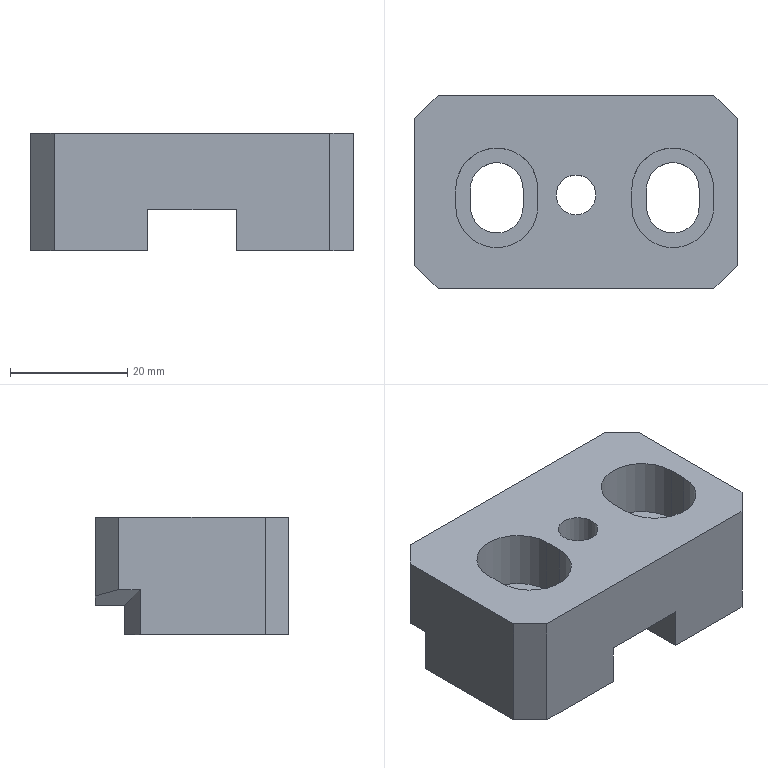Part | NX | features 20 2 | 1 solid | 41 faces | box 55 x 33 x 20 mm | volume 24793 mm3 | plane 32 | cylinder 9 | commonest cylinder face diameters 9 x4 14 x4 6.8 x1
STEP:
#1=CARTESIAN_POINT('',(976.502,-433.5,16.5));
#2=VERTEX_POINT('',#1);
#3=CARTESIAN_POINT('',(962.502,-433.5,16.5));
#4=VERTEX_POINT('',#3);
#5=CARTESIAN_POINT('',(969.502,-433.5,16.5));
#6=DIRECTION('',(0.,0.,1.));
#7=DIRECTION('',(1.,0.,0.));
#8=AXIS2_PLACEMENT_3D('',#5,#6,#7);
#9=CIRCLE('',#8,7.);
#10=EDGE_CURVE('',#2,#4,#9,.T.);
#11=ORIENTED_EDGE('',*,*,#10,.F.);
#12=CARTESIAN_POINT('',(976.502,-436.5,16.5));
#13=VERTEX_POINT('',#12);
#14=CARTESIAN_POINT('',(976.502,-450.5,16.5));
#15=DIRECTION('',(0.,1.,0.));
#16=VECTOR('',#15,1000.);
#17=LINE('',#14,#16);
#18=EDGE_CURVE('',#13,#2,#17,.T.);
#19=ORIENTED_EDGE('',*,*,#18,.F.);
#20=CARTESIAN_POINT('',(962.502,-436.5,16.5));
#21=VERTEX_POINT('',#20);
#22=CARTESIAN_POINT('',(969.502,-436.5,16.5));
#23=DIRECTION('',(0.,0.,1.));
#24=DIRECTION('',(1.,0.,0.));
#25=AXIS2_PLACEMENT_3D('',#22,#23,#24);
#26=CIRCLE('',#25,7.);
#27=EDGE_CURVE('',#21,#13,#26,.T.);
#28=ORIENTED_EDGE('',*,*,#27,.F.);
#29=CARTESIAN_POINT('',(962.502,-450.5,16.5));
#30=DIRECTION('',(0.,-1.,0.));
#31=VECTOR('',#30,1000.);
#32=LINE('',#29,#31);
#33=EDGE_CURVE('',#4,#21,#32,.T.);
#34=ORIENTED_EDGE('',*,*,#33,.F.);
#35=EDGE_LOOP('',(#11,#19,#28,#34));
#36=FACE_BOUND('',#35,.T.);
#37=CARTESIAN_POINT('',(946.502,-436.5,16.5));
#38=VERTEX_POINT('',#37);
#39=CARTESIAN_POINT('',(946.502,-433.5,16.5));
#40=VERTEX_POINT('',#39);
#41=CARTESIAN_POINT('',(946.502,-450.5,16.5));
#42=DIRECTION('',(0.,1.,0.));
#43=VECTOR('',#42,1000.);
#44=LINE('',#41,#43);
#45=EDGE_CURVE('',#38,#40,#44,.T.);
#46=ORIENTED_EDGE('',*,*,#45,.F.);
#47=CARTESIAN_POINT('',(932.502,-436.5,16.5));
#48=VERTEX_POINT('',#47);
#49=CARTESIAN_POINT('',(939.502,-436.5,16.5));
#50=DIRECTION('',(0.,0.,1.));
#51=DIRECTION('',(1.,0.,0.));
#52=AXIS2_PLACEMENT_3D('',#49,#50,#51);
#53=CIRCLE('',#52,7.);
#54=EDGE_CURVE('',#48,#38,#53,.T.);
#55=ORIENTED_EDGE('',*,*,#54,.F.);
#56=CARTESIAN_POINT('',(932.502,-433.5,16.5));
#57=VERTEX_POINT('',#56);
#58=CARTESIAN_POINT('',(932.502,-450.5,16.5));
#59=DIRECTION('',(0.,-1.,0.));
#60=VECTOR('',#59,1000.);
#61=LINE('',#58,#60);
#62=EDGE_CURVE('',#57,#48,#61,.T.);
#63=ORIENTED_EDGE('',*,*,#62,.F.);
#64=CARTESIAN_POINT('',(939.502,-433.5,16.5));
#65=DIRECTION('',(0.,0.,1.));
#66=DIRECTION('',(1.,0.,0.));
#67=AXIS2_PLACEMENT_3D('',#64,#65,#66);
#68=CIRCLE('',#67,7.);
#69=EDGE_CURVE('',#40,#57,#68,.T.);
#70=ORIENTED_EDGE('',*,*,#69,.F.);
#71=EDGE_LOOP('',(#46,#55,#63,#70));
#72=FACE_BOUND('',#71,.T.);
#73=CARTESIAN_POINT('',(976.502,-417.5,16.5));
#74=VERTEX_POINT('',#73);
#75=CARTESIAN_POINT('',(929.502,-417.5,16.5));
#76=VERTEX_POINT('',#75);
#77=CARTESIAN_POINT('',(1043.502,-417.5,16.5));
#78=DIRECTION('',(-1.,0.,0.));
#79=VECTOR('',#78,1000.);
#80=LINE('',#77,#79);
#81=EDGE_CURVE('',#74,#76,#80,.T.);
#82=ORIENTED_EDGE('',*,*,#81,.T.);
#83=CARTESIAN_POINT('',(925.502,-421.5,16.5));
#84=VERTEX_POINT('',#83);
#85=CARTESIAN_POINT('',(925.502,-421.5,16.5));
#86=DIRECTION('',(-0.7071,-0.7071,0.));
#87=VECTOR('',#86,1000.);
#88=LINE('',#85,#87);
#89=EDGE_CURVE('',#76,#84,#88,.T.);
#90=ORIENTED_EDGE('',*,*,#89,.T.);
#91=CARTESIAN_POINT('',(925.502,-446.5,16.5));
#92=VERTEX_POINT('',#91);
#93=CARTESIAN_POINT('',(925.502,-417.5,16.5));
#94=DIRECTION('',(0.,-1.,0.));
#95=VECTOR('',#94,1000.);
#96=LINE('',#93,#95);
#97=EDGE_CURVE('',#84,#92,#96,.T.);
#98=ORIENTED_EDGE('',*,*,#97,.T.);
#99=CARTESIAN_POINT('',(929.502,-450.5,16.5));
#100=VERTEX_POINT('',#99);
#101=CARTESIAN_POINT('',(929.502,-450.5,16.5));
#102=DIRECTION('',(0.7071,-0.7071,0.));
#103=VECTOR('',#102,1000.);
#104=LINE('',#101,#103);
#105=EDGE_CURVE('',#92,#100,#104,.T.);
#106=ORIENTED_EDGE('',*,*,#105,.T.);
#107=CARTESIAN_POINT('',(976.502,-450.5,16.5));
#108=VERTEX_POINT('',#107);
#109=CARTESIAN_POINT('',(963.502,-450.5,16.5));
#110=DIRECTION('',(1.,0.,0.));
#111=VECTOR('',#110,1000.);
#112=LINE('',#109,#111);
#113=EDGE_CURVE('',#100,#108,#112,.T.);
#114=ORIENTED_EDGE('',*,*,#113,.T.);
#115=CARTESIAN_POINT('',(980.502,-446.5,16.5));
#116=VERTEX_POINT('',#115);
#117=CARTESIAN_POINT('',(980.502,-446.5,16.5));
#118=DIRECTION('',(0.7071,0.7071,0.));
#119=VECTOR('',#118,1000.);
#120=LINE('',#117,#119);
#121=EDGE_CURVE('',#108,#116,#120,.T.);
#122=ORIENTED_EDGE('',*,*,#121,.T.);
#123=CARTESIAN_POINT('',(980.502,-421.5,16.5));
#124=VERTEX_POINT('',#123);
#125=CARTESIAN_POINT('',(980.502,-450.5,16.5));
#126=DIRECTION('',(0.,1.,0.));
#127=VECTOR('',#126,1000.);
#128=LINE('',#125,#127);
#129=EDGE_CURVE('',#116,#124,#128,.T.);
#130=ORIENTED_EDGE('',*,*,#129,.T.);
#131=CARTESIAN_POINT('',(976.502,-417.5,16.5));
#132=DIRECTION('',(-0.7071,0.7071,0.));
#133=VECTOR('',#132,1000.);
#134=LINE('',#131,#133);
#135=EDGE_CURVE('',#124,#74,#134,.T.);
#136=ORIENTED_EDGE('',*,*,#135,.T.);
#137=EDGE_LOOP('',(#82,#90,#98,#106,#114,#122,#130,#136));
#138=FACE_BOUND('',#137,.T.);
#139=CARTESIAN_POINT('',(956.402,-434.5,16.5));
#140=VERTEX_POINT('',#139);
#141=CARTESIAN_POINT('',(953.002,-434.5,16.5));
#142=DIRECTION('',(0.,0.,-1.));
#143=DIRECTION('',(1.,0.,0.));
#144=AXIS2_PLACEMENT_3D('',#141,#142,#143);
#145=CIRCLE('',#144,3.4);
#146=EDGE_CURVE('',#140,#140,#145,.T.);
#147=ORIENTED_EDGE('',*,*,#146,.T.);
#148=EDGE_LOOP('',(#147));
#149=FACE_BOUND('',#148,.T.);
#150=CARTESIAN_POINT('',(1043.502,-450.5,16.5));
#151=DIRECTION('',(0.,0.,1.));
#152=DIRECTION('',(-1.,0.,0.));
#153=AXIS2_PLACEMENT_3D('',#150,#151,#152);
#154=PLANE('',#153);
#155=ADVANCED_FACE('',(#36,#72,#138,#149),#154,.T.);
#156=CARTESIAN_POINT('',(965.002,-436.5,6.5));
#157=VERTEX_POINT('',#156);
#158=CARTESIAN_POINT('',(965.002,-433.5,6.5));
#159=VERTEX_POINT('',#158);
#160=CARTESIAN_POINT('',(965.002,-432.5,6.5));
#161=DIRECTION('',(0.,1.,0.));
#162=VECTOR('',#161,1000.);
#163=LINE('',#160,#162);
#164=EDGE_CURVE('',#157,#159,#163,.T.);
#165=ORIENTED_EDGE('',*,*,#164,.T.);
#166=CARTESIAN_POINT('',(974.002,-433.5,6.5));
#167=VERTEX_POINT('',#166);
#168=CARTESIAN_POINT('',(969.502,-433.5,6.5));
#169=DIRECTION('',(0.,0.,-1.));
#170=DIRECTION('',(-1.,0.,0.));
#171=AXIS2_PLACEMENT_3D('',#168,#169,#170);
#172=CIRCLE('',#171,4.5);
#173=EDGE_CURVE('',#159,#167,#172,.T.);
#174=ORIENTED_EDGE('',*,*,#173,.T.);
#175=CARTESIAN_POINT('',(974.002,-436.5,6.5));
#176=VERTEX_POINT('',#175);
#177=CARTESIAN_POINT('',(974.002,-439.5,6.5));
#178=DIRECTION('',(0.,-1.,0.));
#179=VECTOR('',#178,1000.);
#180=LINE('',#177,#179);
#181=EDGE_CURVE('',#167,#176,#180,.T.);
#182=ORIENTED_EDGE('',*,*,#181,.T.);
#183=CARTESIAN_POINT('',(969.502,-436.5,6.5));
#184=DIRECTION('',(0.,0.,-1.));
#185=DIRECTION('',(-1.,0.,0.));
#186=AXIS2_PLACEMENT_3D('',#183,#184,#185);
#187=CIRCLE('',#186,4.5);
#188=EDGE_CURVE('',#176,#157,#187,.T.);
#189=ORIENTED_EDGE('',*,*,#188,.T.);
#190=EDGE_LOOP('',(#165,#174,#182,#189));
#191=FACE_BOUND('',#190,.T.);
#192=CARTESIAN_POINT('',(976.502,-433.5,6.5));
#193=VERTEX_POINT('',#192);
#194=CARTESIAN_POINT('',(962.502,-433.5,6.5));
#195=VERTEX_POINT('',#194);
#196=CARTESIAN_POINT('',(969.502,-433.5,6.5));
#197=DIRECTION('',(0.,0.,1.));
#198=DIRECTION('',(-1.,0.,0.));
#199=AXIS2_PLACEMENT_3D('',#196,#197,#198);
#200=CIRCLE('',#199,7.);
#201=EDGE_CURVE('',#193,#195,#200,.T.);
#202=ORIENTED_EDGE('',*,*,#201,.T.);
#203=CARTESIAN_POINT('',(962.502,-436.5,6.5));
#204=VERTEX_POINT('',#203);
#205=CARTESIAN_POINT('',(962.502,-439.5,6.5));
#206=DIRECTION('',(0.,-1.,0.));
#207=VECTOR('',#206,1000.);
#208=LINE('',#205,#207);
#209=EDGE_CURVE('',#195,#204,#208,.T.);
#210=ORIENTED_EDGE('',*,*,#209,.T.);
#211=CARTESIAN_POINT('',(976.502,-436.5,6.5));
#212=VERTEX_POINT('',#211);
#213=CARTESIAN_POINT('',(969.502,-436.5,6.5));
#214=DIRECTION('',(0.,0.,1.));
#215=DIRECTION('',(-1.,0.,0.));
#216=AXIS2_PLACEMENT_3D('',#213,#214,#215);
#217=CIRCLE('',#216,7.);
#218=EDGE_CURVE('',#204,#212,#217,.T.);
#219=ORIENTED_EDGE('',*,*,#218,.T.);
#220=CARTESIAN_POINT('',(976.502,-432.5,6.5));
#221=DIRECTION('',(0.,1.,0.));
#222=VECTOR('',#221,1000.);
#223=LINE('',#220,#222);
#224=EDGE_CURVE('',#212,#193,#223,.T.);
#225=ORIENTED_EDGE('',*,*,#224,.T.);
#226=EDGE_LOOP('',(#202,#210,#219,#225));
#227=FACE_BOUND('',#226,.T.);
#228=CARTESIAN_POINT('',(969.502,-432.5,6.5));
#229=DIRECTION('',(0.,0.,-1.));
#230=DIRECTION('',(1.,0.,0.));
#231=AXIS2_PLACEMENT_3D('',#228,#229,#230);
#232=PLANE('',#231);
#233=ADVANCED_FACE('',(#191,#227),#232,.F.);
#234=CARTESIAN_POINT('',(970.502,-417.5,1.5));
#235=VERTEX_POINT('',#234);
#236=CARTESIAN_POINT('',(970.502,-422.5,1.5));
#237=VERTEX_POINT('',#236);
#238=CARTESIAN_POINT('',(970.502,-425.18,1.5));
#239=DIRECTION('',(0.,-1.,0.));
#240=VECTOR('',#239,1000.);
#241=LINE('',#238,#240);
#242=EDGE_CURVE('',#235,#237,#241,.T.);
#243=ORIENTED_EDGE('',*,*,#242,.F.);
#244=CARTESIAN_POINT('',(976.502,-417.5,3.108));
#245=VERTEX_POINT('',#244);
#246=CARTESIAN_POINT('',(970.502,-417.5,1.5));
#247=DIRECTION('',(-0.9659,0.,-0.2588));
#248=VECTOR('',#247,1000.);
#249=LINE('',#246,#248);
#250=EDGE_CURVE('',#245,#235,#249,.T.);
#251=ORIENTED_EDGE('',*,*,#250,.F.);
#252=CARTESIAN_POINT('',(980.502,-421.5,4.179));
#253=VERTEX_POINT('',#252);
#254=CARTESIAN_POINT('',(963.451,-404.449,-0.3894));
#255=DIRECTION('',(0.6947,-0.6947,0.1862));
#256=VECTOR('',#255,1000.);
#257=LINE('',#254,#256);
#258=EDGE_CURVE('',#245,#253,#257,.T.);
#259=ORIENTED_EDGE('',*,*,#258,.T.);
#260=CARTESIAN_POINT('',(980.502,-425.18,4.179));
#261=VERTEX_POINT('',#260);
#262=CARTESIAN_POINT('',(980.502,-417.5,4.179));
#263=DIRECTION('',(0.,1.,0.));
#264=VECTOR('',#263,1000.);
#265=LINE('',#262,#264);
#266=EDGE_CURVE('',#261,#253,#265,.T.);
#267=ORIENTED_EDGE('',*,*,#266,.F.);
#268=CARTESIAN_POINT('',(979.875,-425.012,4.011));
#269=DIRECTION('',(0.9351,-0.2506,0.2506));
#270=VECTOR('',#269,1000.);
#271=LINE('',#268,#270);
#272=EDGE_CURVE('',#237,#261,#271,.T.);
#273=ORIENTED_EDGE('',*,*,#272,.F.);
#274=EDGE_LOOP('',(#243,#251,#259,#267,#273));
#275=FACE_BOUND('',#274,.T.);
#276=CARTESIAN_POINT('',(970.502,-396.891,1.5));
#277=DIRECTION('',(0.2588,0.,-0.9659));
#278=DIRECTION('',(0.9659,0.,0.2588));
#279=AXIS2_PLACEMENT_3D('',#276,#277,#278);
#280=PLANE('',#279);
#281=ADVANCED_FACE('',(#275),#280,.T.);
#282=CARTESIAN_POINT('',(944.002,-433.5,6.5));
#283=VERTEX_POINT('',#282);
#284=CARTESIAN_POINT('',(944.002,-436.5,6.5));
#285=VERTEX_POINT('',#284);
#286=CARTESIAN_POINT('',(944.002,-432.5,6.5));
#287=DIRECTION('',(0.,-1.,0.));
#288=VECTOR('',#287,1000.);
#289=LINE('',#286,#288);
#290=EDGE_CURVE('',#283,#285,#289,.T.);
#291=ORIENTED_EDGE('',*,*,#290,.T.);
#292=CARTESIAN_POINT('',(935.002,-436.5,6.5));
#293=VERTEX_POINT('',#292);
#294=CARTESIAN_POINT('',(939.502,-436.5,6.5));
#295=DIRECTION('',(0.,0.,-1.));
#296=DIRECTION('',(-1.,0.,0.));
#297=AXIS2_PLACEMENT_3D('',#294,#295,#296);
#298=CIRCLE('',#297,4.5);
#299=EDGE_CURVE('',#285,#293,#298,.T.);
#300=ORIENTED_EDGE('',*,*,#299,.T.);
#301=CARTESIAN_POINT('',(935.002,-433.5,6.5));
#302=VERTEX_POINT('',#301);
#303=CARTESIAN_POINT('',(935.002,-439.5,6.5));
#304=DIRECTION('',(0.,1.,0.));
#305=VECTOR('',#304,1000.);
#306=LINE('',#303,#305);
#307=EDGE_CURVE('',#293,#302,#306,.T.);
#308=ORIENTED_EDGE('',*,*,#307,.T.);
#309=CARTESIAN_POINT('',(939.502,-433.5,6.5));
#310=DIRECTION('',(0.,0.,-1.));
#311=DIRECTION('',(-1.,0.,0.));
#312=AXIS2_PLACEMENT_3D('',#309,#310,#311);
#313=CIRCLE('',#312,4.5);
#314=EDGE_CURVE('',#302,#283,#313,.T.);
#315=ORIENTED_EDGE('',*,*,#314,.T.);
#316=EDGE_LOOP('',(#291,#300,#308,#315));
#317=FACE_BOUND('',#316,.T.);
#318=CARTESIAN_POINT('',(946.502,-433.5,6.5));
#319=VERTEX_POINT('',#318);
#320=CARTESIAN_POINT('',(932.502,-433.5,6.5));
#321=VERTEX_POINT('',#320);
#322=CARTESIAN_POINT('',(939.502,-433.5,6.5));
#323=DIRECTION('',(0.,0.,1.));
#324=DIRECTION('',(-1.,0.,0.));
#325=AXIS2_PLACEMENT_3D('',#322,#323,#324);
#326=CIRCLE('',#325,7.);
#327=EDGE_CURVE('',#319,#321,#326,.T.);
#328=ORIENTED_EDGE('',*,*,#327,.T.);
#329=CARTESIAN_POINT('',(932.502,-436.5,6.5));
#330=VERTEX_POINT('',#329);
#331=CARTESIAN_POINT('',(932.502,-432.5,6.5));
#332=DIRECTION('',(0.,-1.,0.));
#333=VECTOR('',#332,1000.);
#334=LINE('',#331,#333);
#335=EDGE_CURVE('',#321,#330,#334,.T.);
#336=ORIENTED_EDGE('',*,*,#335,.T.);
#337=CARTESIAN_POINT('',(946.502,-436.5,6.5));
#338=VERTEX_POINT('',#337);
#339=CARTESIAN_POINT('',(939.502,-436.5,6.5));
#340=DIRECTION('',(0.,0.,1.));
#341=DIRECTION('',(-1.,0.,0.));
#342=AXIS2_PLACEMENT_3D('',#339,#340,#341);
#343=CIRCLE('',#342,7.);
#344=EDGE_CURVE('',#330,#338,#343,.T.);
#345=ORIENTED_EDGE('',*,*,#344,.T.);
#346=CARTESIAN_POINT('',(946.502,-439.5,6.5));
#347=DIRECTION('',(0.,1.,0.));
#348=VECTOR('',#347,1000.);
#349=LINE('',#346,#348);
#350=EDGE_CURVE('',#338,#319,#349,.T.);
#351=ORIENTED_EDGE('',*,*,#350,.T.);
#352=EDGE_LOOP('',(#328,#336,#345,#351));
#353=FACE_BOUND('',#352,.T.);
#354=CARTESIAN_POINT('',(939.502,-432.5,6.5));
#355=DIRECTION('',(0.,0.,-1.));
#356=DIRECTION('',(-1.,0.,0.));
#357=AXIS2_PLACEMENT_3D('',#354,#355,#356);
#358=PLANE('',#357);
#359=ADVANCED_FACE('',(#317,#353),#358,.F.);
#360=ORIENTED_EDGE('',*,*,#33,.T.);
#361=CARTESIAN_POINT('',(962.502,-436.5,42.5));
#362=DIRECTION('',(0.,0.,1.));
#363=VECTOR('',#362,1000.);
#364=LINE('',#361,#363);
#365=EDGE_CURVE('',#204,#21,#364,.T.);
#366=ORIENTED_EDGE('',*,*,#365,.F.);
#367=ORIENTED_EDGE('',*,*,#209,.F.);
#368=CARTESIAN_POINT('',(962.502,-433.5,42.5));
#369=DIRECTION('',(0.,0.,1.));
#370=VECTOR('',#369,1000.);
#371=LINE('',#368,#370);
#372=EDGE_CURVE('',#195,#4,#371,.T.);
#373=ORIENTED_EDGE('',*,*,#372,.T.);
#374=EDGE_LOOP('',(#360,#366,#367,#373));
#375=FACE_BOUND('',#374,.T.);
#376=CARTESIAN_POINT('',(962.502,-439.5,42.5));
#377=DIRECTION('',(-1.,0.,0.));
#378=DIRECTION('',(0.,0.,-1.));
#379=AXIS2_PLACEMENT_3D('',#376,#377,#378);
#380=PLANE('',#379);
#381=ADVANCED_FACE('',(#375),#380,.F.);
#382=ORIENTED_EDGE('',*,*,#27,.T.);
#383=CARTESIAN_POINT('',(976.502,-436.5,42.5));
#384=DIRECTION('',(0.,0.,1.));
#385=VECTOR('',#384,1000.);
#386=LINE('',#383,#385);
#387=EDGE_CURVE('',#212,#13,#386,.T.);
#388=ORIENTED_EDGE('',*,*,#387,.F.);
#389=ORIENTED_EDGE('',*,*,#218,.F.);
#390=ORIENTED_EDGE('',*,*,#365,.T.);
#391=EDGE_LOOP('',(#382,#388,#389,#390));
#392=FACE_BOUND('',#391,.T.);
#393=CARTESIAN_POINT('',(969.502,-436.5,42.5));
#394=DIRECTION('',(0.,0.,-1.));
#395=DIRECTION('',(1.,0.,0.));
#396=AXIS2_PLACEMENT_3D('',#393,#394,#395);
#397=CYLINDRICAL_SURFACE('',#396,7.);
#398=ADVANCED_FACE('',(#392),#397,.F.);
#399=ORIENTED_EDGE('',*,*,#18,.T.);
#400=CARTESIAN_POINT('',(976.502,-433.5,42.5));
#401=DIRECTION('',(0.,0.,1.));
#402=VECTOR('',#401,1000.);
#403=LINE('',#400,#402);
#404=EDGE_CURVE('',#193,#2,#403,.T.);
#405=ORIENTED_EDGE('',*,*,#404,.F.);
#406=ORIENTED_EDGE('',*,*,#224,.F.);
#407=ORIENTED_EDGE('',*,*,#387,.T.);
#408=EDGE_LOOP('',(#399,#405,#406,#407));
#409=FACE_BOUND('',#408,.T.);
#410=CARTESIAN_POINT('',(976.502,-432.5,42.5));
#411=DIRECTION('',(1.,0.,0.));
#412=DIRECTION('',(0.,0.,1.));
#413=AXIS2_PLACEMENT_3D('',#410,#411,#412);
#414=PLANE('',#413);
#415=ADVANCED_FACE('',(#409),#414,.F.);
#416=ORIENTED_EDGE('',*,*,#10,.T.);
#417=ORIENTED_EDGE('',*,*,#372,.F.);
#418=ORIENTED_EDGE('',*,*,#201,.F.);
#419=ORIENTED_EDGE('',*,*,#404,.T.);
#420=EDGE_LOOP('',(#416,#417,#418,#419));
#421=FACE_BOUND('',#420,.T.);
#422=CARTESIAN_POINT('',(969.502,-433.5,42.5));
#423=DIRECTION('',(0.,0.,-1.));
#424=DIRECTION('',(1.,0.,0.));
#425=AXIS2_PLACEMENT_3D('',#422,#423,#424);
#426=CYLINDRICAL_SURFACE('',#425,7.);
#427=ADVANCED_FACE('',(#421),#426,.F.);
#428=ORIENTED_EDGE('',*,*,#135,.F.);
#429=CARTESIAN_POINT('',(980.502,-421.5,11.5));
#430=DIRECTION('',(0.,0.,1.));
#431=VECTOR('',#430,1000.);
#432=LINE('',#429,#431);
#433=EDGE_CURVE('',#253,#124,#432,.T.);
#434=ORIENTED_EDGE('',*,*,#433,.F.);
#435=ORIENTED_EDGE('',*,*,#258,.F.);
#436=CARTESIAN_POINT('',(976.502,-417.5,11.5));
#437=DIRECTION('',(0.,0.,-1.));
#438=VECTOR('',#437,1000.);
#439=LINE('',#436,#438);
#440=EDGE_CURVE('',#74,#245,#439,.T.);
#441=ORIENTED_EDGE('',*,*,#440,.F.);
#442=EDGE_LOOP('',(#428,#434,#435,#441));
#443=FACE_BOUND('',#442,.T.);
#444=CARTESIAN_POINT('',(976.502,-417.5,11.5));
#445=DIRECTION('',(-0.7071,-0.7071,0.));
#446=DIRECTION('',(0.,0.,-1.));
#447=AXIS2_PLACEMENT_3D('',#444,#445,#446);
#448=PLANE('',#447);
#449=ADVANCED_FACE('',(#443),#448,.F.);
#450=ORIENTED_EDGE('',*,*,#69,.T.);
#451=CARTESIAN_POINT('',(932.502,-433.5,42.5));
#452=DIRECTION('',(0.,0.,-1.));
#453=VECTOR('',#452,1000.);
#454=LINE('',#451,#453);
#455=EDGE_CURVE('',#57,#321,#454,.T.);
#456=ORIENTED_EDGE('',*,*,#455,.T.);
#457=ORIENTED_EDGE('',*,*,#327,.F.);
#458=CARTESIAN_POINT('',(946.502,-433.5,42.5));
#459=DIRECTION('',(0.,0.,-1.));
#460=VECTOR('',#459,1000.);
#461=LINE('',#458,#460);
#462=EDGE_CURVE('',#40,#319,#461,.T.);
#463=ORIENTED_EDGE('',*,*,#462,.F.);
#464=EDGE_LOOP('',(#450,#456,#457,#463));
#465=FACE_BOUND('',#464,.T.);
#466=CARTESIAN_POINT('',(939.502,-433.5,42.5));
#467=DIRECTION('',(0.,0.,-1.));
#468=DIRECTION('',(-1.,0.,0.));
#469=AXIS2_PLACEMENT_3D('',#466,#467,#468);
#470=CYLINDRICAL_SURFACE('',#469,7.);
#471=ADVANCED_FACE('',(#465),#470,.F.);
#472=ORIENTED_EDGE('',*,*,#62,.T.);
#473=CARTESIAN_POINT('',(932.502,-436.5,42.5));
#474=DIRECTION('',(0.,0.,-1.));
#475=VECTOR('',#474,1000.);
#476=LINE('',#473,#475);
#477=EDGE_CURVE('',#48,#330,#476,.T.);
#478=ORIENTED_EDGE('',*,*,#477,.T.);
#479=ORIENTED_EDGE('',*,*,#335,.F.);
#480=ORIENTED_EDGE('',*,*,#455,.F.);
#481=EDGE_LOOP('',(#472,#478,#479,#480));
#482=FACE_BOUND('',#481,.T.);
#483=CARTESIAN_POINT('',(932.502,-432.5,42.5));
#484=DIRECTION('',(-1.,0.,0.));
#485=DIRECTION('',(0.,0.,1.));
#486=AXIS2_PLACEMENT_3D('',#483,#484,#485);
#487=PLANE('',#486);
#488=ADVANCED_FACE('',(#482),#487,.F.);
#489=ORIENTED_EDGE('',*,*,#54,.T.);
#490=CARTESIAN_POINT('',(946.502,-436.5,42.5));
#491=DIRECTION('',(0.,0.,-1.));
#492=VECTOR('',#491,1000.);
#493=LINE('',#490,#492);
#494=EDGE_CURVE('',#38,#338,#493,.T.);
#495=ORIENTED_EDGE('',*,*,#494,.T.);
#496=ORIENTED_EDGE('',*,*,#344,.F.);
#497=ORIENTED_EDGE('',*,*,#477,.F.);
#498=EDGE_LOOP('',(#489,#495,#496,#497));
#499=FACE_BOUND('',#498,.T.);
#500=CARTESIAN_POINT('',(939.502,-436.5,42.5));
#501=DIRECTION('',(0.,0.,-1.));
#502=DIRECTION('',(-1.,0.,0.));
#503=AXIS2_PLACEMENT_3D('',#500,#501,#502);
#504=CYLINDRICAL_SURFACE('',#503,7.);
#505=ADVANCED_FACE('',(#499),#504,.F.);
#506=ORIENTED_EDGE('',*,*,#45,.T.);
#507=ORIENTED_EDGE('',*,*,#462,.T.);
#508=ORIENTED_EDGE('',*,*,#350,.F.);
#509=ORIENTED_EDGE('',*,*,#494,.F.);
#510=EDGE_LOOP('',(#506,#507,#508,#509));
#511=FACE_BOUND('',#510,.T.);
#512=CARTESIAN_POINT('',(946.502,-439.5,42.5));
#513=DIRECTION('',(1.,0.,0.));
#514=DIRECTION('',(0.,0.,-1.));
#515=AXIS2_PLACEMENT_3D('',#512,#513,#514);
#516=PLANE('',#515);
#517=ADVANCED_FACE('',(#511),#516,.F.);
#518=ORIENTED_EDGE('',*,*,#266,.T.);
#519=ORIENTED_EDGE('',*,*,#433,.T.);
#520=ORIENTED_EDGE('',*,*,#129,.F.);
#521=CARTESIAN_POINT('',(980.502,-446.5,-3.5));
#522=VERTEX_POINT('',#521);
#523=CARTESIAN_POINT('',(980.502,-446.5,11.5));
#524=DIRECTION('',(0.,0.,-1.));
#525=VECTOR('',#524,1000.);
#526=LINE('',#523,#525);
#527=EDGE_CURVE('',#116,#522,#526,.T.);
#528=ORIENTED_EDGE('',*,*,#527,.T.);
#529=CARTESIAN_POINT('',(980.502,-425.18,-3.5));
#530=VERTEX_POINT('',#529);
#531=CARTESIAN_POINT('',(980.502,-450.5,-3.5));
#532=DIRECTION('',(0.,1.,0.));
#533=VECTOR('',#532,1000.);
#534=LINE('',#531,#533);
#535=EDGE_CURVE('',#522,#530,#534,.T.);
#536=ORIENTED_EDGE('',*,*,#535,.T.);
#537=CARTESIAN_POINT('',(980.502,-425.18,3.5));
#538=DIRECTION('',(0.,0.,-1.));
#539=VECTOR('',#538,1000.);
#540=LINE('',#537,#539);
#541=EDGE_CURVE('',#261,#530,#540,.T.);
#542=ORIENTED_EDGE('',*,*,#541,.F.);
#543=EDGE_LOOP('',(#518,#519,#520,#528,#536,#542));
#544=FACE_BOUND('',#543,.T.);
#545=CARTESIAN_POINT('',(980.502,-450.5,11.5));
#546=DIRECTION('',(-1.,0.,0.));
#547=DIRECTION('',(0.,0.,-1.));
#548=AXIS2_PLACEMENT_3D('',#545,#546,#547);
#549=PLANE('',#548);
#550=ADVANCED_FACE('',(#544),#549,.F.);
#551=CARTESIAN_POINT('',(970.501,-422.5,1.5));
#552=VERTEX_POINT('',#551);
#553=CARTESIAN_POINT('',(980.502,-425.18,1.5));
#554=DIRECTION('',(0.9659,-0.2588,0.));
#555=VECTOR('',#554,1000.);
#556=LINE('',#553,#555);
#557=EDGE_CURVE('',#552,#237,#556,.T.);
#558=ORIENTED_EDGE('',*,*,#557,.T.);
#559=ORIENTED_EDGE('',*,*,#272,.T.);
#560=ORIENTED_EDGE('',*,*,#541,.T.);
#561=CARTESIAN_POINT('',(970.501,-422.5,-3.5));
#562=VERTEX_POINT('',#561);
#563=CARTESIAN_POINT('',(980.502,-425.18,-3.5));
#564=DIRECTION('',(-0.9659,0.2588,0.));
#565=VECTOR('',#564,1000.);
#566=LINE('',#563,#565);
#567=EDGE_CURVE('',#530,#562,#566,.T.);
#568=ORIENTED_EDGE('',*,*,#567,.T.);
#569=CARTESIAN_POINT('',(970.501,-422.5,3.5));
#570=DIRECTION('',(0.,0.,1.));
#571=VECTOR('',#570,1000.);
#572=LINE('',#569,#571);
#573=EDGE_CURVE('',#562,#552,#572,.T.);
#574=ORIENTED_EDGE('',*,*,#573,.T.);
#575=EDGE_LOOP('',(#558,#559,#560,#568,#574));
#576=FACE_BOUND('',#575,.T.);
#577=CARTESIAN_POINT('',(980.502,-425.18,3.5));
#578=DIRECTION('',(-0.2588,-0.9659,0.));
#579=DIRECTION('',(0.9659,-0.2588,0.));
#580=AXIS2_PLACEMENT_3D('',#577,#578,#579);
#581=PLANE('',#580);
#582=ADVANCED_FACE('',(#576),#581,.F.);
#583=ORIENTED_EDGE('',*,*,#173,.F.);
#584=CARTESIAN_POINT('',(965.002,-433.5,-3.5));
#585=VERTEX_POINT('',#584);
#586=CARTESIAN_POINT('',(965.002,-433.5,42.5));
#587=DIRECTION('',(0.,0.,1.));
#588=VECTOR('',#587,1000.);
#589=LINE('',#586,#588);
#590=EDGE_CURVE('',#585,#159,#589,.T.);
#591=ORIENTED_EDGE('',*,*,#590,.F.);
#592=CARTESIAN_POINT('',(974.002,-433.5,-3.5));
#593=VERTEX_POINT('',#592);
#594=CARTESIAN_POINT('',(969.502,-433.5,-3.5));
#595=DIRECTION('',(0.,0.,1.));
#596=DIRECTION('',(1.,0.,0.));
#597=AXIS2_PLACEMENT_3D('',#594,#595,#596);
#598=CIRCLE('',#597,4.5);
#599=EDGE_CURVE('',#593,#585,#598,.T.);
#600=ORIENTED_EDGE('',*,*,#599,.F.);
#601=CARTESIAN_POINT('',(974.002,-433.5,42.5));
#602=DIRECTION('',(0.,0.,1.));
#603=VECTOR('',#602,1000.);
#604=LINE('',#601,#603);
#605=EDGE_CURVE('',#593,#167,#604,.T.);
#606=ORIENTED_EDGE('',*,*,#605,.T.);
#607=EDGE_LOOP('',(#583,#591,#600,#606));
#608=FACE_BOUND('',#607,.T.);
#609=CARTESIAN_POINT('',(969.502,-433.5,42.5));
#610=DIRECTION('',(0.,0.,-1.));
#611=DIRECTION('',(1.,0.,0.));
#612=AXIS2_PLACEMENT_3D('',#609,#610,#611);
#613=CYLINDRICAL_SURFACE('',#612,4.5);
#614=ADVANCED_FACE('',(#608),#613,.F.);
#615=ORIENTED_EDGE('',*,*,#181,.F.);
#616=ORIENTED_EDGE('',*,*,#605,.F.);
#617=CARTESIAN_POINT('',(974.002,-436.5,-3.5));
#618=VERTEX_POINT('',#617);
#619=CARTESIAN_POINT('',(974.002,-439.5,-3.5));
#620=DIRECTION('',(0.,1.,0.));
#621=VECTOR('',#620,1000.);
#622=LINE('',#619,#621);
#623=EDGE_CURVE('',#618,#593,#622,.T.);
#624=ORIENTED_EDGE('',*,*,#623,.F.);
#625=CARTESIAN_POINT('',(974.002,-436.5,42.5));
#626=DIRECTION('',(0.,0.,1.));
#627=VECTOR('',#626,1000.);
#628=LINE('',#625,#627);
#629=EDGE_CURVE('',#618,#176,#628,.T.);
#630=ORIENTED_EDGE('',*,*,#629,.T.);
#631=EDGE_LOOP('',(#615,#616,#624,#630));
#632=FACE_BOUND('',#631,.T.);
#633=CARTESIAN_POINT('',(974.002,-439.5,42.5));
#634=DIRECTION('',(-1.,0.,0.));
#635=DIRECTION('',(0.,0.,-1.));
#636=AXIS2_PLACEMENT_3D('',#633,#634,#635);
#637=PLANE('',#636);
#638=ADVANCED_FACE('',(#632),#637,.T.);
#639=ORIENTED_EDGE('',*,*,#188,.F.);
#640=ORIENTED_EDGE('',*,*,#629,.F.);
#641=CARTESIAN_POINT('',(965.002,-436.5,-3.5));
#642=VERTEX_POINT('',#641);
#643=CARTESIAN_POINT('',(969.502,-436.5,-3.5));
#644=DIRECTION('',(0.,0.,1.));
#645=DIRECTION('',(1.,0.,0.));
#646=AXIS2_PLACEMENT_3D('',#643,#644,#645);
#647=CIRCLE('',#646,4.5);
#648=EDGE_CURVE('',#642,#618,#647,.T.);
#649=ORIENTED_EDGE('',*,*,#648,.F.);
#650=CARTESIAN_POINT('',(965.002,-436.5,42.5));
#651=DIRECTION('',(0.,0.,1.));
#652=VECTOR('',#651,1000.);
#653=LINE('',#650,#652);
#654=EDGE_CURVE('',#642,#157,#653,.T.);
#655=ORIENTED_EDGE('',*,*,#654,.T.);
#656=EDGE_LOOP('',(#639,#640,#649,#655));
#657=FACE_BOUND('',#656,.T.);
#658=CARTESIAN_POINT('',(969.502,-436.5,42.5));
#659=DIRECTION('',(0.,0.,-1.));
#660=DIRECTION('',(1.,0.,0.));
#661=AXIS2_PLACEMENT_3D('',#658,#659,#660);
#662=CYLINDRICAL_SURFACE('',#661,4.5);
#663=ADVANCED_FACE('',(#657),#662,.F.);
#664=ORIENTED_EDGE('',*,*,#164,.F.);
#665=ORIENTED_EDGE('',*,*,#654,.F.);
#666=CARTESIAN_POINT('',(965.002,-432.5,-3.5));
#667=DIRECTION('',(0.,-1.,0.));
#668=VECTOR('',#667,1000.);
#669=LINE('',#666,#668);
#670=EDGE_CURVE('',#585,#642,#669,.T.);
#671=ORIENTED_EDGE('',*,*,#670,.F.);
#672=ORIENTED_EDGE('',*,*,#590,.T.);
#673=EDGE_LOOP('',(#664,#665,#671,#672));
#674=FACE_BOUND('',#673,.T.);
#675=CARTESIAN_POINT('',(965.002,-432.5,42.5));
#676=DIRECTION('',(1.,0.,0.));
#677=DIRECTION('',(0.,0.,1.));
#678=AXIS2_PLACEMENT_3D('',#675,#676,#677);
#679=PLANE('',#678);
#680=ADVANCED_FACE('',(#674),#679,.T.);
#681=CARTESIAN_POINT('',(960.502,-422.5,-3.5));
#682=VERTEX_POINT('',#681);
#683=CARTESIAN_POINT('',(960.502,-422.5,1.5));
#684=VERTEX_POINT('',#683);
#685=CARTESIAN_POINT('',(960.502,-422.5,-9.5));
#686=DIRECTION('',(0.,0.,1.));
#687=VECTOR('',#686,1000.);
#688=LINE('',#685,#687);
#689=EDGE_CURVE('',#682,#684,#688,.T.);
#690=ORIENTED_EDGE('',*,*,#689,.T.);
#691=CARTESIAN_POINT('',(895.773,-422.5,1.5));
#692=DIRECTION('',(1.,0.,0.));
#693=VECTOR('',#692,1000.);
#694=LINE('',#691,#693);
#695=EDGE_CURVE('',#684,#552,#694,.T.);
#696=ORIENTED_EDGE('',*,*,#695,.T.);
#697=ORIENTED_EDGE('',*,*,#573,.F.);
#698=CARTESIAN_POINT('',(913.501,-422.5,-3.5));
#699=DIRECTION('',(-1.,0.,0.));
#700=VECTOR('',#699,1000.);
#701=LINE('',#698,#700);
#702=EDGE_CURVE('',#562,#682,#701,.T.);
#703=ORIENTED_EDGE('',*,*,#702,.T.);
#704=EDGE_LOOP('',(#690,#696,#697,#703));
#705=FACE_BOUND('',#704,.T.);
#706=CARTESIAN_POINT('',(913.501,-422.5,3.5));
#707=DIRECTION('',(0.,-1.,0.));
#708=DIRECTION('',(0.,0.,1.));
#709=AXIS2_PLACEMENT_3D('',#706,#707,#708);
#710=PLANE('',#709);
#711=ADVANCED_FACE('',(#705),#710,.F.);
#712=CARTESIAN_POINT('',(960.502,-417.5,1.5));
#713=VERTEX_POINT('',#712);
#714=CARTESIAN_POINT('',(960.502,-436.5,1.5));
#715=DIRECTION('',(0.,1.,0.));
#716=VECTOR('',#715,1000.);
#717=LINE('',#714,#716);
#718=EDGE_CURVE('',#684,#713,#717,.T.);
#719=ORIENTED_EDGE('',*,*,#718,.T.);
#720=CARTESIAN_POINT('',(873.502,-417.5,1.5));
#721=DIRECTION('',(1.,0.,0.));
#722=VECTOR('',#721,1000.);
#723=LINE('',#720,#722);
#724=EDGE_CURVE('',#713,#235,#723,.T.);
#725=ORIENTED_EDGE('',*,*,#724,.T.);
#726=ORIENTED_EDGE('',*,*,#242,.T.);
#727=ORIENTED_EDGE('',*,*,#557,.F.);
#728=ORIENTED_EDGE('',*,*,#695,.F.);
#729=EDGE_LOOP('',(#719,#725,#726,#727,#728));
#730=FACE_BOUND('',#729,.T.);
#731=CARTESIAN_POINT('',(945.773,-396.891,1.5));
#732=DIRECTION('',(0.,0.,-1.));
#733=DIRECTION('',(1.,0.,0.));
#734=AXIS2_PLACEMENT_3D('',#731,#732,#733);
#735=PLANE('',#734);
#736=ADVANCED_FACE('',(#730),#735,.T.);
#737=CARTESIAN_POINT('',(945.502,-417.5,1.5));
#738=VERTEX_POINT('',#737);
#739=CARTESIAN_POINT('',(945.502,-417.5,3.5));
#740=VERTEX_POINT('',#739);
#741=CARTESIAN_POINT('',(945.502,-417.5,11.5));
#742=DIRECTION('',(0.,0.,1.));
#743=VECTOR('',#742,1000.);
#744=LINE('',#741,#743);
#745=EDGE_CURVE('',#738,#740,#744,.T.);
#746=ORIENTED_EDGE('',*,*,#745,.F.);
#747=CARTESIAN_POINT('',(935.502,-417.5,1.5));
#748=VERTEX_POINT('',#747);
#749=CARTESIAN_POINT('',(1021.502,-417.5,1.5));
#750=DIRECTION('',(1.,0.,0.));
#751=VECTOR('',#750,1000.);
#752=LINE('',#749,#751);
#753=EDGE_CURVE('',#748,#738,#752,.T.);
#754=ORIENTED_EDGE('',*,*,#753,.F.);
#755=CARTESIAN_POINT('',(929.502,-417.5,3.108));
#756=VERTEX_POINT('',#755);
#757=CARTESIAN_POINT('',(935.502,-417.5,1.5));
#758=DIRECTION('',(-0.9659,0.,0.2588));
#759=VECTOR('',#758,1000.);
#760=LINE('',#757,#759);
#761=EDGE_CURVE('',#748,#756,#760,.T.);
#762=ORIENTED_EDGE('',*,*,#761,.T.);
#763=CARTESIAN_POINT('',(929.502,-417.5,11.5));
#764=DIRECTION('',(0.,0.,1.));
#765=VECTOR('',#764,1000.);
#766=LINE('',#763,#765);
#767=EDGE_CURVE('',#756,#76,#766,.T.);
#768=ORIENTED_EDGE('',*,*,#767,.T.);
#769=ORIENTED_EDGE('',*,*,#81,.F.);
#770=ORIENTED_EDGE('',*,*,#440,.T.);
#771=ORIENTED_EDGE('',*,*,#250,.T.);
#772=ORIENTED_EDGE('',*,*,#724,.F.);
#773=CARTESIAN_POINT('',(960.502,-417.5,3.5));
#774=VERTEX_POINT('',#773);
#775=CARTESIAN_POINT('',(960.502,-417.5,11.5));
#776=DIRECTION('',(0.,0.,-1.));
#777=VECTOR('',#776,1000.);
#778=LINE('',#775,#777);
#779=EDGE_CURVE('',#774,#713,#778,.T.);
#780=ORIENTED_EDGE('',*,*,#779,.F.);
#781=CARTESIAN_POINT('',(936.002,-417.5,3.5));
#782=DIRECTION('',(1.,0.,0.));
#783=VECTOR('',#782,1000.);
#784=LINE('',#781,#783);
#785=EDGE_CURVE('',#740,#774,#784,.T.);
#786=ORIENTED_EDGE('',*,*,#785,.F.);
#787=EDGE_LOOP('',(#746,#754,#762,#768,#769,#770,#771,#772,#780,#786));
#788=FACE_BOUND('',#787,.T.);
#789=CARTESIAN_POINT('',(1043.502,-417.5,11.5));
#790=DIRECTION('',(0.,-1.,0.));
#791=DIRECTION('',(0.,0.,1.));
#792=AXIS2_PLACEMENT_3D('',#789,#790,#791);
#793=PLANE('',#792);
#794=ADVANCED_FACE('',(#788),#793,.F.);
#795=ORIENTED_EDGE('',*,*,#89,.F.);
#796=ORIENTED_EDGE('',*,*,#767,.F.);
#797=CARTESIAN_POINT('',(925.502,-421.5,4.179));
#798=VERTEX_POINT('',#797);
#799=CARTESIAN_POINT('',(942.554,-404.449,-0.3894));
#800=DIRECTION('',(0.6947,0.6947,-0.1862));
#801=VECTOR('',#800,1000.);
#802=LINE('',#799,#801);
#803=EDGE_CURVE('',#798,#756,#802,.T.);
#804=ORIENTED_EDGE('',*,*,#803,.F.);
#805=CARTESIAN_POINT('',(925.502,-421.5,11.5));
#806=DIRECTION('',(0.,0.,-1.));
#807=VECTOR('',#806,1000.);
#808=LINE('',#805,#807);
#809=EDGE_CURVE('',#84,#798,#808,.T.);
#810=ORIENTED_EDGE('',*,*,#809,.F.);
#811=EDGE_LOOP('',(#795,#796,#804,#810));
#812=FACE_BOUND('',#811,.T.);
#813=CARTESIAN_POINT('',(925.502,-421.5,11.5));
#814=DIRECTION('',(0.7071,-0.7071,0.));
#815=DIRECTION('',(0.,0.,-1.));
#816=AXIS2_PLACEMENT_3D('',#813,#814,#815);
#817=PLANE('',#816);
#818=ADVANCED_FACE('',(#812),#817,.F.);
#819=ORIENTED_EDGE('',*,*,#299,.F.);
#820=CARTESIAN_POINT('',(944.002,-436.5,-3.5));
#821=VERTEX_POINT('',#820);
#822=CARTESIAN_POINT('',(944.002,-436.5,42.5));
#823=DIRECTION('',(0.,0.,-1.));
#824=VECTOR('',#823,1000.);
#825=LINE('',#822,#824);
#826=EDGE_CURVE('',#285,#821,#825,.T.);
#827=ORIENTED_EDGE('',*,*,#826,.T.);
#828=CARTESIAN_POINT('',(935.002,-436.5,-3.5));
#829=VERTEX_POINT('',#828);
#830=CARTESIAN_POINT('',(939.502,-436.5,-3.5));
#831=DIRECTION('',(0.,0.,-1.));
#832=DIRECTION('',(1.,0.,0.));
#833=AXIS2_PLACEMENT_3D('',#830,#831,#832);
#834=CIRCLE('',#833,4.5);
#835=EDGE_CURVE('',#821,#829,#834,.T.);
#836=ORIENTED_EDGE('',*,*,#835,.T.);
#837=CARTESIAN_POINT('',(935.002,-436.5,42.5));
#838=DIRECTION('',(0.,0.,-1.));
#839=VECTOR('',#838,1000.);
#840=LINE('',#837,#839);
#841=EDGE_CURVE('',#293,#829,#840,.T.);
#842=ORIENTED_EDGE('',*,*,#841,.F.);
#843=EDGE_LOOP('',(#819,#827,#836,#842));
#844=FACE_BOUND('',#843,.T.);
#845=CARTESIAN_POINT('',(939.502,-436.5,42.5));
#846=DIRECTION('',(0.,0.,-1.));
#847=DIRECTION('',(-1.,0.,0.));
#848=AXIS2_PLACEMENT_3D('',#845,#846,#847);
#849=CYLINDRICAL_SURFACE('',#848,4.5);
#850=ADVANCED_FACE('',(#844),#849,.F.);
#851=ORIENTED_EDGE('',*,*,#307,.F.);
#852=ORIENTED_EDGE('',*,*,#841,.T.);
#853=CARTESIAN_POINT('',(935.002,-433.5,-3.5));
#854=VERTEX_POINT('',#853);
#855=CARTESIAN_POINT('',(935.002,-450.5,-3.5));
#856=DIRECTION('',(0.,1.,0.));
#857=VECTOR('',#856,1000.);
#858=LINE('',#855,#857);
#859=EDGE_CURVE('',#829,#854,#858,.T.);
#860=ORIENTED_EDGE('',*,*,#859,.T.);
#861=CARTESIAN_POINT('',(935.002,-433.5,42.5));
#862=DIRECTION('',(0.,0.,-1.));
#863=VECTOR('',#862,1000.);
#864=LINE('',#861,#863);
#865=EDGE_CURVE('',#302,#854,#864,.T.);
#866=ORIENTED_EDGE('',*,*,#865,.F.);
#867=EDGE_LOOP('',(#851,#852,#860,#866));
#868=FACE_BOUND('',#867,.T.);
#869=CARTESIAN_POINT('',(935.002,-439.5,42.5));
#870=DIRECTION('',(1.,0.,0.));
#871=DIRECTION('',(0.,0.,-1.));
#872=AXIS2_PLACEMENT_3D('',#869,#870,#871);
#873=PLANE('',#872);
#874=ADVANCED_FACE('',(#868),#873,.T.);
#875=ORIENTED_EDGE('',*,*,#314,.F.);
#876=ORIENTED_EDGE('',*,*,#865,.T.);
#877=CARTESIAN_POINT('',(944.002,-433.5,-3.5));
#878=VERTEX_POINT('',#877);
#879=CARTESIAN_POINT('',(939.502,-433.5,-3.5));
#880=DIRECTION('',(0.,0.,-1.));
#881=DIRECTION('',(1.,0.,0.));
#882=AXIS2_PLACEMENT_3D('',#879,#880,#881);
#883=CIRCLE('',#882,4.5);
#884=EDGE_CURVE('',#854,#878,#883,.T.);
#885=ORIENTED_EDGE('',*,*,#884,.T.);
#886=CARTESIAN_POINT('',(944.002,-433.5,42.5));
#887=DIRECTION('',(0.,0.,-1.));
#888=VECTOR('',#887,1000.);
#889=LINE('',#886,#888);
#890=EDGE_CURVE('',#283,#878,#889,.T.);
#891=ORIENTED_EDGE('',*,*,#890,.F.);
#892=EDGE_LOOP('',(#875,#876,#885,#891));
#893=FACE_BOUND('',#892,.T.);
#894=CARTESIAN_POINT('',(939.502,-433.5,42.5));
#895=DIRECTION('',(0.,0.,-1.));
#896=DIRECTION('',(-1.,0.,0.));
#897=AXIS2_PLACEMENT_3D('',#894,#895,#896);
#898=CYLINDRICAL_SURFACE('',#897,4.5);
#899=ADVANCED_FACE('',(#893),#898,.F.);
#900=ORIENTED_EDGE('',*,*,#290,.F.);
#901=ORIENTED_EDGE('',*,*,#890,.T.);
#902=CARTESIAN_POINT('',(944.002,-450.5,-3.5));
#903=DIRECTION('',(0.,-1.,0.));
#904=VECTOR('',#903,1000.);
#905=LINE('',#902,#904);
#906=EDGE_CURVE('',#878,#821,#905,.T.);
#907=ORIENTED_EDGE('',*,*,#906,.T.);
#908=ORIENTED_EDGE('',*,*,#826,.F.);
#909=EDGE_LOOP('',(#900,#901,#907,#908));
#910=FACE_BOUND('',#909,.T.);
#911=CARTESIAN_POINT('',(944.002,-432.5,42.5));
#912=DIRECTION('',(-1.,0.,0.));
#913=DIRECTION('',(0.,0.,1.));
#914=AXIS2_PLACEMENT_3D('',#911,#912,#913);
#915=PLANE('',#914);
#916=ADVANCED_FACE('',(#910),#915,.T.);
#917=ORIENTED_EDGE('',*,*,#97,.F.);
#918=ORIENTED_EDGE('',*,*,#809,.T.);
#919=CARTESIAN_POINT('',(925.502,-425.179,4.179));
#920=VERTEX_POINT('',#919);
#921=CARTESIAN_POINT('',(925.502,-425.179,4.179));
#922=DIRECTION('',(0.,-1.,0.));
#923=VECTOR('',#922,1000.);
#924=LINE('',#921,#923);
#925=EDGE_CURVE('',#798,#920,#924,.T.);
#926=ORIENTED_EDGE('',*,*,#925,.T.);
#927=CARTESIAN_POINT('',(925.502,-425.179,-3.5));
#928=VERTEX_POINT('',#927);
#929=CARTESIAN_POINT('',(925.502,-425.179,3.5));
#930=DIRECTION('',(0.,0.,-1.));
#931=VECTOR('',#930,1000.);
#932=LINE('',#929,#931);
#933=EDGE_CURVE('',#920,#928,#932,.T.);
#934=ORIENTED_EDGE('',*,*,#933,.T.);
#935=CARTESIAN_POINT('',(925.502,-446.5,-3.5));
#936=VERTEX_POINT('',#935);
#937=CARTESIAN_POINT('',(925.502,-417.5,-3.5));
#938=DIRECTION('',(0.,-1.,0.));
#939=VECTOR('',#938,1000.);
#940=LINE('',#937,#939);
#941=EDGE_CURVE('',#928,#936,#940,.T.);
#942=ORIENTED_EDGE('',*,*,#941,.T.);
#943=CARTESIAN_POINT('',(925.502,-446.5,11.5));
#944=DIRECTION('',(0.,0.,1.));
#945=VECTOR('',#944,1000.);
#946=LINE('',#943,#945);
#947=EDGE_CURVE('',#936,#92,#946,.T.);
#948=ORIENTED_EDGE('',*,*,#947,.T.);
#949=EDGE_LOOP('',(#917,#918,#926,#934,#942,#948));
#950=FACE_BOUND('',#949,.T.);
#951=CARTESIAN_POINT('',(925.502,-417.5,11.5));
#952=DIRECTION('',(1.,0.,0.));
#953=DIRECTION('',(0.,0.,1.));
#954=AXIS2_PLACEMENT_3D('',#951,#952,#953);
#955=PLANE('',#954);
#956=ADVANCED_FACE('',(#950),#955,.F.);
#957=ORIENTED_EDGE('',*,*,#925,.F.);
#958=ORIENTED_EDGE('',*,*,#803,.T.);
#959=ORIENTED_EDGE('',*,*,#761,.F.);
#960=CARTESIAN_POINT('',(935.502,-422.5,1.5));
#961=VERTEX_POINT('',#960);
#962=CARTESIAN_POINT('',(935.502,-417.5,1.5));
#963=DIRECTION('',(0.,1.,0.));
#964=VECTOR('',#963,1000.);
#965=LINE('',#962,#964);
#966=EDGE_CURVE('',#961,#748,#965,.T.);
#967=ORIENTED_EDGE('',*,*,#966,.F.);
#968=CARTESIAN_POINT('',(935.501,-422.5,1.5));
#969=VERTEX_POINT('',#968);
#970=CARTESIAN_POINT('',(935.502,-422.5,1.5));
#971=DIRECTION('',(0.9659,0.,-0.2588));
#972=VECTOR('',#971,1000.);
#973=LINE('',#970,#972);
#974=EDGE_CURVE('',#969,#961,#973,.T.);
#975=ORIENTED_EDGE('',*,*,#974,.F.);
#976=CARTESIAN_POINT('',(935.501,-422.5,1.5));
#977=DIRECTION('',(0.9351,0.2506,-0.2506));
#978=VECTOR('',#977,1000.);
#979=LINE('',#976,#978);
#980=EDGE_CURVE('',#920,#969,#979,.T.);
#981=ORIENTED_EDGE('',*,*,#980,.F.);
#982=EDGE_LOOP('',(#957,#958,#959,#967,#975,#981));
#983=FACE_BOUND('',#982,.T.);
#984=CARTESIAN_POINT('',(935.502,-396.891,1.5));
#985=DIRECTION('',(-0.2588,0.,-0.9659));
#986=DIRECTION('',(0.9659,0.,-0.2588));
#987=AXIS2_PLACEMENT_3D('',#984,#985,#986);
#988=PLANE('',#987);
#989=ADVANCED_FACE('',(#983),#988,.T.);
#990=CARTESIAN_POINT('',(935.501,-422.5,-3.5));
#991=VERTEX_POINT('',#990);
#992=CARTESIAN_POINT('',(935.501,-422.5,-3.5));
#993=DIRECTION('',(-0.9659,-0.2588,0.));
#994=VECTOR('',#993,1000.);
#995=LINE('',#992,#994);
#996=EDGE_CURVE('',#991,#928,#995,.T.);
#997=ORIENTED_EDGE('',*,*,#996,.T.);
#998=ORIENTED_EDGE('',*,*,#933,.F.);
#999=ORIENTED_EDGE('',*,*,#980,.T.);
#1000=CARTESIAN_POINT('',(935.501,-422.5,3.5));
#1001=DIRECTION('',(0.,0.,1.));
#1002=VECTOR('',#1001,1000.);
#1003=LINE('',#1000,#1002);
#1004=EDGE_CURVE('',#991,#969,#1003,.T.);
#1005=ORIENTED_EDGE('',*,*,#1004,.F.);
#1006=EDGE_LOOP('',(#997,#998,#999,#1005));
#1007=FACE_BOUND('',#1006,.T.);
#1008=CARTESIAN_POINT('',(935.501,-422.5,3.5));
#1009=DIRECTION('',(0.2588,-0.9659,0.));
#1010=DIRECTION('',(0.9659,0.2588,0.));
#1011=AXIS2_PLACEMENT_3D('',#1008,#1009,#1010);
#1012=PLANE('',#1011);
#1013=ADVANCED_FACE('',(#1007),#1012,.F.);
#1014=ORIENTED_EDGE('',*,*,#996,.F.);
#1015=CARTESIAN_POINT('',(945.502,-422.5,-3.5));
#1016=VERTEX_POINT('',#1015);
#1017=CARTESIAN_POINT('',(981.501,-422.5,-3.5));
#1018=DIRECTION('',(-1.,0.,0.));
#1019=VECTOR('',#1018,1000.);
#1020=LINE('',#1017,#1019);
#1021=EDGE_CURVE('',#1016,#991,#1020,.T.);
#1022=ORIENTED_EDGE('',*,*,#1021,.F.);
#1023=CARTESIAN_POINT('',(945.502,-450.5,-3.5));
#1024=VERTEX_POINT('',#1023);
#1025=CARTESIAN_POINT('',(945.502,-450.5,-3.5));
#1026=DIRECTION('',(0.,-1.,0.));
#1027=VECTOR('',#1026,1000.);
#1028=LINE('',#1025,#1027);
#1029=EDGE_CURVE('',#1016,#1024,#1028,.T.);
#1030=ORIENTED_EDGE('',*,*,#1029,.T.);
#1031=CARTESIAN_POINT('',(929.502,-450.5,-3.5));
#1032=VERTEX_POINT('',#1031);
#1033=CARTESIAN_POINT('',(1003.502,-450.5,-3.5));
#1034=DIRECTION('',(1.,0.,0.));
#1035=VECTOR('',#1034,1000.);
#1036=LINE('',#1033,#1035);
#1037=EDGE_CURVE('',#1032,#1024,#1036,.T.);
#1038=ORIENTED_EDGE('',*,*,#1037,.F.);
#1039=CARTESIAN_POINT('',(929.502,-450.5,-3.5));
#1040=DIRECTION('',(-0.7071,0.7071,0.));
#1041=VECTOR('',#1040,1000.);
#1042=LINE('',#1039,#1041);
#1043=EDGE_CURVE('',#1032,#936,#1042,.T.);
#1044=ORIENTED_EDGE('',*,*,#1043,.T.);
#1045=ORIENTED_EDGE('',*,*,#941,.F.);
#1046=EDGE_LOOP('',(#1014,#1022,#1030,#1038,#1044,#1045));
#1047=FACE_BOUND('',#1046,.T.);
#1048=ORIENTED_EDGE('',*,*,#906,.F.);
#1049=ORIENTED_EDGE('',*,*,#884,.F.);
#1050=ORIENTED_EDGE('',*,*,#859,.F.);
#1051=ORIENTED_EDGE('',*,*,#835,.F.);
#1052=EDGE_LOOP('',(#1048,#1049,#1050,#1051));
#1053=FACE_BOUND('',#1052,.T.);
#1054=CARTESIAN_POINT('',(1073.502,-450.5,-3.5));
#1055=DIRECTION('',(0.,0.,1.));
#1056=DIRECTION('',(-1.,0.,0.));
#1057=AXIS2_PLACEMENT_3D('',#1054,#1055,#1056);
#1058=PLANE('',#1057);
#1059=ADVANCED_FACE('',(#1047,#1053),#1058,.F.);
#1060=ORIENTED_EDGE('',*,*,#1043,.F.);
#1061=CARTESIAN_POINT('',(929.502,-450.5,11.5));
#1062=DIRECTION('',(0.,0.,-1.));
#1063=VECTOR('',#1062,1000.);
#1064=LINE('',#1061,#1063);
#1065=EDGE_CURVE('',#100,#1032,#1064,.T.);
#1066=ORIENTED_EDGE('',*,*,#1065,.F.);
#1067=ORIENTED_EDGE('',*,*,#105,.F.);
#1068=ORIENTED_EDGE('',*,*,#947,.F.);
#1069=EDGE_LOOP('',(#1060,#1066,#1067,#1068));
#1070=FACE_BOUND('',#1069,.T.);
#1071=CARTESIAN_POINT('',(929.502,-450.5,11.5));
#1072=DIRECTION('',(0.7071,0.7071,0.));
#1073=DIRECTION('',(0.,0.,-1.));
#1074=AXIS2_PLACEMENT_3D('',#1071,#1072,#1073);
#1075=PLANE('',#1074);
#1076=ADVANCED_FACE('',(#1070),#1075,.F.);
#1077=CARTESIAN_POINT('',(976.502,-450.5,-3.5));
#1078=VERTEX_POINT('',#1077);
#1079=CARTESIAN_POINT('',(980.502,-446.5,-3.5));
#1080=DIRECTION('',(-0.7071,-0.7071,0.));
#1081=VECTOR('',#1080,1000.);
#1082=LINE('',#1079,#1081);
#1083=EDGE_CURVE('',#522,#1078,#1082,.T.);
#1084=ORIENTED_EDGE('',*,*,#1083,.F.);
#1085=ORIENTED_EDGE('',*,*,#527,.F.);
#1086=ORIENTED_EDGE('',*,*,#121,.F.);
#1087=CARTESIAN_POINT('',(976.502,-450.5,11.5));
#1088=DIRECTION('',(0.,0.,1.));
#1089=VECTOR('',#1088,1000.);
#1090=LINE('',#1087,#1089);
#1091=EDGE_CURVE('',#1078,#108,#1090,.T.);
#1092=ORIENTED_EDGE('',*,*,#1091,.F.);
#1093=EDGE_LOOP('',(#1084,#1085,#1086,#1092));
#1094=FACE_BOUND('',#1093,.T.);
#1095=CARTESIAN_POINT('',(980.502,-446.5,11.5));
#1096=DIRECTION('',(-0.7071,0.7071,0.));
#1097=DIRECTION('',(0.,0.,-1.));
#1098=AXIS2_PLACEMENT_3D('',#1095,#1096,#1097);
#1099=PLANE('',#1098);
#1100=ADVANCED_FACE('',(#1094),#1099,.F.);
#1101=ORIENTED_EDGE('',*,*,#670,.T.);
#1102=ORIENTED_EDGE('',*,*,#648,.T.);
#1103=ORIENTED_EDGE('',*,*,#623,.T.);
#1104=ORIENTED_EDGE('',*,*,#599,.T.);
#1105=EDGE_LOOP('',(#1101,#1102,#1103,#1104));
#1106=FACE_BOUND('',#1105,.T.);
#1107=ORIENTED_EDGE('',*,*,#702,.F.);
#1108=ORIENTED_EDGE('',*,*,#567,.F.);
#1109=ORIENTED_EDGE('',*,*,#535,.F.);
#1110=ORIENTED_EDGE('',*,*,#1083,.T.);
#1111=CARTESIAN_POINT('',(960.502,-450.5,-3.5));
#1112=VERTEX_POINT('',#1111);
#1113=CARTESIAN_POINT('',(843.502,-450.5,-3.5));
#1114=DIRECTION('',(1.,0.,0.));
#1115=VECTOR('',#1114,1000.);
#1116=LINE('',#1113,#1115);
#1117=EDGE_CURVE('',#1112,#1078,#1116,.T.);
#1118=ORIENTED_EDGE('',*,*,#1117,.F.);
#1119=CARTESIAN_POINT('',(960.502,-450.5,-3.5));
#1120=DIRECTION('',(0.,1.,0.));
#1121=VECTOR('',#1120,1000.);
#1122=LINE('',#1119,#1121);
#1123=EDGE_CURVE('',#1112,#682,#1122,.T.);
#1124=ORIENTED_EDGE('',*,*,#1123,.T.);
#1125=EDGE_LOOP('',(#1107,#1108,#1109,#1110,#1118,#1124));
#1126=FACE_BOUND('',#1125,.T.);
#1127=CARTESIAN_POINT('',(863.502,-450.5,-3.5));
#1128=DIRECTION('',(0.,0.,1.));
#1129=DIRECTION('',(-1.,0.,0.));
#1130=AXIS2_PLACEMENT_3D('',#1127,#1128,#1129);
#1131=PLANE('',#1130);
#1132=ADVANCED_FACE('',(#1106,#1126),#1131,.F.);
#1133=ORIENTED_EDGE('',*,*,#1123,.F.);
#1134=CARTESIAN_POINT('',(960.502,-450.5,3.5));
#1135=VERTEX_POINT('',#1134);
#1136=CARTESIAN_POINT('',(960.502,-450.5,-9.5));
#1137=DIRECTION('',(0.,0.,1.));
#1138=VECTOR('',#1137,1000.);
#1139=LINE('',#1136,#1138);
#1140=EDGE_CURVE('',#1112,#1135,#1139,.T.);
#1141=ORIENTED_EDGE('',*,*,#1140,.T.);
#1142=CARTESIAN_POINT('',(960.502,-436.5,3.5));
#1143=DIRECTION('',(0.,-1.,0.));
#1144=VECTOR('',#1143,1000.);
#1145=LINE('',#1142,#1144);
#1146=EDGE_CURVE('',#774,#1135,#1145,.T.);
#1147=ORIENTED_EDGE('',*,*,#1146,.F.);
#1148=ORIENTED_EDGE('',*,*,#779,.T.);
#1149=ORIENTED_EDGE('',*,*,#718,.F.);
#1150=ORIENTED_EDGE('',*,*,#689,.F.);
#1151=EDGE_LOOP('',(#1133,#1141,#1147,#1148,#1149,#1150));
#1152=FACE_BOUND('',#1151,.T.);
#1153=CARTESIAN_POINT('',(960.502,-436.5,-9.5));
#1154=DIRECTION('',(1.,0.,0.));
#1155=DIRECTION('',(0.,0.,-1.));
#1156=AXIS2_PLACEMENT_3D('',#1153,#1154,#1155);
#1157=PLANE('',#1156);
#1158=ADVANCED_FACE('',(#1152),#1157,.F.);
#1159=CARTESIAN_POINT('',(956.402,-434.5,3.5));
#1160=VERTEX_POINT('',#1159);
#1161=CARTESIAN_POINT('',(953.002,-434.5,3.5));
#1162=DIRECTION('',(0.,0.,1.));
#1163=DIRECTION('',(1.,0.,0.));
#1164=AXIS2_PLACEMENT_3D('',#1161,#1162,#1163);
#1165=CIRCLE('',#1164,3.4);
#1166=EDGE_CURVE('',#1160,#1160,#1165,.T.);
#1167=ORIENTED_EDGE('',*,*,#1166,.T.);
#1168=EDGE_LOOP('',(#1167));
#1169=FACE_BOUND('',#1168,.T.);
#1170=CARTESIAN_POINT('',(945.502,-450.5,3.5));
#1171=VERTEX_POINT('',#1170);
#1172=CARTESIAN_POINT('',(856.002,-450.5,3.5));
#1173=DIRECTION('',(1.,0.,0.));
#1174=VECTOR('',#1173,1000.);
#1175=LINE('',#1172,#1174);
#1176=EDGE_CURVE('',#1171,#1135,#1175,.T.);
#1177=ORIENTED_EDGE('',*,*,#1176,.F.);
#1178=CARTESIAN_POINT('',(945.502,-436.5,3.5));
#1179=DIRECTION('',(0.,1.,0.));
#1180=VECTOR('',#1179,1000.);
#1181=LINE('',#1178,#1180);
#1182=EDGE_CURVE('',#1171,#740,#1181,.T.);
#1183=ORIENTED_EDGE('',*,*,#1182,.T.);
#1184=ORIENTED_EDGE('',*,*,#785,.T.);
#1185=ORIENTED_EDGE('',*,*,#1146,.T.);
#1186=EDGE_LOOP('',(#1177,#1183,#1184,#1185));
#1187=FACE_BOUND('',#1186,.T.);
#1188=CARTESIAN_POINT('',(953.002,-436.5,3.5));
#1189=DIRECTION('',(0.,0.,1.));
#1190=DIRECTION('',(0.,-1.,0.));
#1191=AXIS2_PLACEMENT_3D('',#1188,#1189,#1190);
#1192=PLANE('',#1191);
#1193=ADVANCED_FACE('',(#1169,#1187),#1192,.F.);
#1194=ORIENTED_EDGE('',*,*,#1182,.F.);
#1195=CARTESIAN_POINT('',(945.502,-450.5,11.5));
#1196=DIRECTION('',(0.,0.,1.));
#1197=VECTOR('',#1196,1000.);
#1198=LINE('',#1195,#1197);
#1199=EDGE_CURVE('',#1024,#1171,#1198,.T.);
#1200=ORIENTED_EDGE('',*,*,#1199,.F.);
#1201=ORIENTED_EDGE('',*,*,#1029,.F.);
#1202=CARTESIAN_POINT('',(945.502,-422.5,1.5));
#1203=VERTEX_POINT('',#1202);
#1204=CARTESIAN_POINT('',(945.502,-422.5,3.5));
#1205=DIRECTION('',(0.,0.,-1.));
#1206=VECTOR('',#1205,1000.);
#1207=LINE('',#1204,#1206);
#1208=EDGE_CURVE('',#1203,#1016,#1207,.T.);
#1209=ORIENTED_EDGE('',*,*,#1208,.F.);
#1210=CARTESIAN_POINT('',(945.502,-396.891,1.5));
#1211=DIRECTION('',(0.,1.,0.));
#1212=VECTOR('',#1211,1000.);
#1213=LINE('',#1210,#1212);
#1214=EDGE_CURVE('',#1203,#738,#1213,.T.);
#1215=ORIENTED_EDGE('',*,*,#1214,.T.);
#1216=ORIENTED_EDGE('',*,*,#745,.T.);
#1217=EDGE_LOOP('',(#1194,#1200,#1201,#1209,#1215,#1216));
#1218=FACE_BOUND('',#1217,.T.);
#1219=CARTESIAN_POINT('',(945.502,-436.5,0.));
#1220=DIRECTION('',(1.,0.,0.));
#1221=DIRECTION('',(0.,0.,1.));
#1222=AXIS2_PLACEMENT_3D('',#1219,#1220,#1221);
#1223=PLANE('',#1222);
#1224=ADVANCED_FACE('',(#1218),#1223,.T.);
#1225=ORIENTED_EDGE('',*,*,#1037,.T.);
#1226=ORIENTED_EDGE('',*,*,#1199,.T.);
#1227=ORIENTED_EDGE('',*,*,#1176,.T.);
#1228=ORIENTED_EDGE('',*,*,#1140,.F.);
#1229=ORIENTED_EDGE('',*,*,#1117,.T.);
#1230=ORIENTED_EDGE('',*,*,#1091,.T.);
#1231=ORIENTED_EDGE('',*,*,#113,.F.);
#1232=ORIENTED_EDGE('',*,*,#1065,.T.);
#1233=EDGE_LOOP('',(#1225,#1226,#1227,#1228,#1229,#1230,#1231,#1232));
#1234=FACE_BOUND('',#1233,.T.);
#1235=CARTESIAN_POINT('',(963.502,-450.5,11.5));
#1236=DIRECTION('',(0.,1.,0.));
#1237=DIRECTION('',(0.,0.,-1.));
#1238=AXIS2_PLACEMENT_3D('',#1235,#1236,#1237);
#1239=PLANE('',#1238);
#1240=ADVANCED_FACE('',(#1234),#1239,.F.);
#1241=ORIENTED_EDGE('',*,*,#753,.T.);
#1242=ORIENTED_EDGE('',*,*,#1214,.F.);
#1243=CARTESIAN_POINT('',(1011.501,-422.5,1.5));
#1244=DIRECTION('',(1.,0.,0.));
#1245=VECTOR('',#1244,1000.);
#1246=LINE('',#1243,#1245);
#1247=EDGE_CURVE('',#961,#1203,#1246,.T.);
#1248=ORIENTED_EDGE('',*,*,#1247,.F.);
#1249=ORIENTED_EDGE('',*,*,#966,.T.);
#1250=EDGE_LOOP('',(#1241,#1242,#1248,#1249));
#1251=FACE_BOUND('',#1250,.T.);
#1252=CARTESIAN_POINT('',(1043.773,-396.891,1.5));
#1253=DIRECTION('',(0.,0.,-1.));
#1254=DIRECTION('',(1.,0.,0.));
#1255=AXIS2_PLACEMENT_3D('',#1252,#1253,#1254);
#1256=PLANE('',#1255);
#1257=ADVANCED_FACE('',(#1251),#1256,.T.);
#1258=ORIENTED_EDGE('',*,*,#1247,.T.);
#1259=ORIENTED_EDGE('',*,*,#1208,.T.);
#1260=ORIENTED_EDGE('',*,*,#1021,.T.);
#1261=ORIENTED_EDGE('',*,*,#1004,.T.);
#1262=ORIENTED_EDGE('',*,*,#974,.T.);
#1263=EDGE_LOOP('',(#1258,#1259,#1260,#1261,#1262));
#1264=FACE_BOUND('',#1263,.T.);
#1265=CARTESIAN_POINT('',(1011.501,-422.5,3.5));
#1266=DIRECTION('',(0.,-1.,0.));
#1267=DIRECTION('',(0.,0.,1.));
#1268=AXIS2_PLACEMENT_3D('',#1265,#1266,#1267);
#1269=PLANE('',#1268);
#1270=ADVANCED_FACE('',(#1264),#1269,.F.);
#1271=ORIENTED_EDGE('',*,*,#146,.F.);
#1272=EDGE_LOOP('',(#1271));
#1273=FACE_BOUND('',#1272,.T.);
#1274=ORIENTED_EDGE('',*,*,#1166,.F.);
#1275=EDGE_LOOP('',(#1274));
#1276=FACE_BOUND('',#1275,.T.);
#1277=CARTESIAN_POINT('',(953.002,-434.5,16.5));
#1278=DIRECTION('',(0.,0.,-1.));
#1279=DIRECTION('',(-1.,0.,0.));
#1280=AXIS2_PLACEMENT_3D('',#1277,#1278,#1279);
#1281=CYLINDRICAL_SURFACE('',#1280,3.4);
#1282=ADVANCED_FACE('',(#1273,#1276),#1281,.F.);
#1283=CLOSED_SHELL('',(#155,#233,#281,#359,#381,#398,#415,#427,#449,#471,#488,#505,#517,#550,#582,#614,#638,#663,#680,#711,#736,#794,#818,#850,#874,#899,#916,#956,#989,#1013,#1059,#1076,#1100,#1132,#1158,#1193,#1224,#1240,#1257,#1270,#1282));
#1284=MANIFOLD_SOLID_BREP('',#1283);
#1285=(LENGTH_UNIT()NAMED_UNIT(*)SI_UNIT(.MILLI.,.METRE.));
#1286=UNCERTAINTY_MEASURE_WITH_UNIT(LENGTH_MEASURE(0.00001),#1285,'','');
#1287=(NAMED_UNIT(*)PLANE_ANGLE_UNIT()SI_UNIT($,.RADIAN.));
#1288=(NAMED_UNIT(*)SI_UNIT($,.STERADIAN.)SOLID_ANGLE_UNIT());
#1289=(GEOMETRIC_REPRESENTATION_CONTEXT(3)GLOBAL_UNCERTAINTY_ASSIGNED_CONTEXT((#1286))GLOBAL_UNIT_ASSIGNED_CONTEXT((#1285,#1287,#1288))REPRESENTATION_CONTEXT('',''));
#1290=ADVANCED_BREP_SHAPE_REPRESENTATION('',(#1284),#1289);